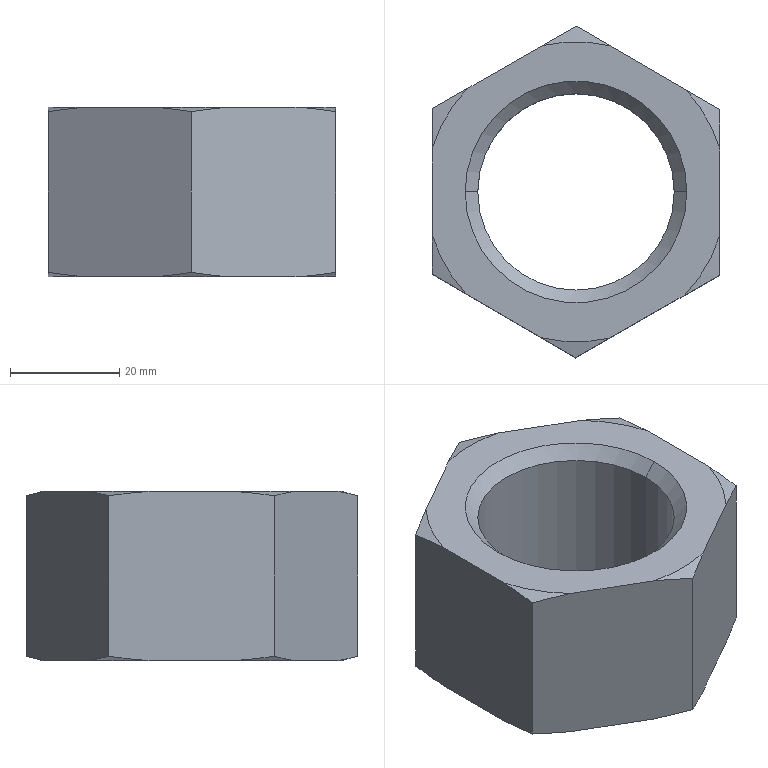Part | SolidWorks | features Cut 2, Chamfer 1, Extrusion 1 | 1 solid | 26 faces | box 52.765 x 60.79 x 31 mm | volume 42176 mm3 | cone 16 | plane 8 | cylinder 2 | commonest cylinder face diameters 36 x2
STEP:
#1=CARTESIAN_POINT('',(-18.,0.,28.693));
#2=VERTEX_POINT('',#1);
#3=CARTESIAN_POINT('',(18.,0.,28.693));
#4=VERTEX_POINT('',#3);
#5=CARTESIAN_POINT('',(0.,0.,28.693));
#6=DIRECTION('',(0.,0.,1.));
#7=DIRECTION('',(-1.,0.,0.));
#8=AXIS2_PLACEMENT_3D('',#5,#6,#7);
#9=CIRCLE('',#8,18.);
#10=EDGE_CURVE('',#2,#4,#9,.T.);
#11=ORIENTED_EDGE('',*,*,#10,.F.);
#12=CARTESIAN_POINT('',(-20.307,0.,31.));
#13=VERTEX_POINT('',#12);
#14=CARTESIAN_POINT('',(-18.,0.,28.693));
#15=DIRECTION('',(-0.7071,0.,0.7071));
#16=VECTOR('',#15,1000.);
#17=LINE('',#14,#16);
#18=EDGE_CURVE('',#2,#13,#17,.T.);
#19=ORIENTED_EDGE('',*,*,#18,.T.);
#20=CARTESIAN_POINT('',(20.307,0.,31.));
#21=VERTEX_POINT('',#20);
#22=CARTESIAN_POINT('',(0.,0.,31.));
#23=DIRECTION('',(0.,0.,-1.));
#24=DIRECTION('',(-1.,0.,0.));
#25=AXIS2_PLACEMENT_3D('',#22,#23,#24);
#26=CIRCLE('',#25,20.307);
#27=EDGE_CURVE('',#21,#13,#26,.T.);
#28=ORIENTED_EDGE('',*,*,#27,.F.);
#29=CARTESIAN_POINT('',(18.,0.,28.693));
#30=DIRECTION('',(0.7071,0.,0.7071));
#31=VECTOR('',#30,1000.);
#32=LINE('',#29,#31);
#33=EDGE_CURVE('',#4,#21,#32,.T.);
#34=ORIENTED_EDGE('',*,*,#33,.F.);
#35=EDGE_LOOP('',(#11,#19,#28,#34));
#36=FACE_OUTER_BOUND('',#35,.T.);
#37=CARTESIAN_POINT('',(0.,0.,28.693));
#38=DIRECTION('',(0.,0.,1.));
#39=DIRECTION('',(1.,0.,0.));
#40=AXIS2_PLACEMENT_3D('',#37,#38,#39);
#41=CONICAL_SURFACE('',#40,18.,0.7854);
#42=ADVANCED_FACE('',(#36),#41,.F.);
#43=CARTESIAN_POINT('',(18.,0.,2.307));
#44=VERTEX_POINT('',#43);
#45=CARTESIAN_POINT('',(-18.,0.,2.307));
#46=VERTEX_POINT('',#45);
#47=CARTESIAN_POINT('',(0.,0.,2.307));
#48=DIRECTION('',(0.,0.,-1.));
#49=DIRECTION('',(-1.,0.,0.));
#50=AXIS2_PLACEMENT_3D('',#47,#48,#49);
#51=CIRCLE('',#50,18.);
#52=EDGE_CURVE('',#44,#46,#51,.T.);
#53=ORIENTED_EDGE('',*,*,#52,.F.);
#54=CARTESIAN_POINT('',(20.307,0.,0.));
#55=VERTEX_POINT('',#54);
#56=CARTESIAN_POINT('',(20.307,0.,0.));
#57=DIRECTION('',(0.7071,0.,-0.7071));
#58=VECTOR('',#57,1000.);
#59=LINE('',#56,#58);
#60=EDGE_CURVE('',#44,#55,#59,.T.);
#61=ORIENTED_EDGE('',*,*,#60,.T.);
#62=CARTESIAN_POINT('',(-20.307,0.,0.));
#63=VERTEX_POINT('',#62);
#64=CARTESIAN_POINT('',(0.,0.,0.));
#65=DIRECTION('',(0.,0.,1.));
#66=DIRECTION('',(-1.,0.,0.));
#67=AXIS2_PLACEMENT_3D('',#64,#65,#66);
#68=CIRCLE('',#67,20.307);
#69=EDGE_CURVE('',#63,#55,#68,.T.);
#70=ORIENTED_EDGE('',*,*,#69,.F.);
#71=CARTESIAN_POINT('',(-20.307,0.,0.));
#72=DIRECTION('',(-0.7071,0.,-0.7071));
#73=VECTOR('',#72,1000.);
#74=LINE('',#71,#73);
#75=EDGE_CURVE('',#46,#63,#74,.T.);
#76=ORIENTED_EDGE('',*,*,#75,.F.);
#77=EDGE_LOOP('',(#53,#61,#70,#76));
#78=FACE_OUTER_BOUND('',#77,.T.);
#79=CARTESIAN_POINT('',(0.,0.,0.));
#80=DIRECTION('',(0.,0.,-1.));
#81=DIRECTION('',(-1.,0.,0.));
#82=AXIS2_PLACEMENT_3D('',#79,#80,#81);
#83=CONICAL_SURFACE('',#82,20.307,0.7854);
#84=ADVANCED_FACE('',(#78),#83,.F.);
#85=ORIENTED_EDGE('',*,*,#10,.T.);
#86=CARTESIAN_POINT('',(18.,0.,31.));
#87=DIRECTION('',(0.,0.,-1.));
#88=VECTOR('',#87,1000.);
#89=LINE('',#86,#88);
#90=EDGE_CURVE('',#4,#44,#89,.T.);
#91=ORIENTED_EDGE('',*,*,#90,.T.);
#92=ORIENTED_EDGE('',*,*,#52,.T.);
#93=CARTESIAN_POINT('',(-18.,0.,31.));
#94=DIRECTION('',(0.,0.,-1.));
#95=VECTOR('',#94,1000.);
#96=LINE('',#93,#95);
#97=EDGE_CURVE('',#2,#46,#96,.T.);
#98=ORIENTED_EDGE('',*,*,#97,.F.);
#99=EDGE_LOOP('',(#85,#91,#92,#98));
#100=FACE_OUTER_BOUND('',#99,.T.);
#101=CARTESIAN_POINT('',(0.,0.,31.));
#102=DIRECTION('',(0.,0.,-1.));
#103=DIRECTION('',(-1.,0.,0.));
#104=AXIS2_PLACEMENT_3D('',#101,#102,#103);
#105=CYLINDRICAL_SURFACE('',#104,18.);
#106=ADVANCED_FACE('',(#100),#105,.F.);
#107=CARTESIAN_POINT('',(26.382,15.094,30.224));
#108=VERTEX_POINT('',#107);
#109=CARTESIAN_POINT('',(20.129,18.737,31.));
#110=VERTEX_POINT('',#109);
#111=CARTESIAN_POINT('',(26.382,15.094,30.224));
#112=CARTESIAN_POINT('',(24.305,16.304,30.546));
#113=CARTESIAN_POINT('',(22.221,17.518,30.812));
#114=CARTESIAN_POINT('',(20.129,18.737,31.));
#115=B_SPLINE_CURVE_WITH_KNOTS('',3,(#111,#112,#113,#114),.UNSPECIFIED.,.F.,.F.,(4,4),(0.03012,0.0374),.UNSPECIFIED.);
#116=EDGE_CURVE('',#108,#110,#115,.T.);
#117=ORIENTED_EDGE('',*,*,#116,.F.);
#118=CARTESIAN_POINT('',(26.382,15.094,0.7757));
#119=VERTEX_POINT('',#118);
#120=CARTESIAN_POINT('',(26.382,15.094,31.));
#121=DIRECTION('',(0.,0.,-1.));
#122=VECTOR('',#121,1000.);
#123=LINE('',#120,#122);
#124=EDGE_CURVE('',#108,#119,#123,.T.);
#125=ORIENTED_EDGE('',*,*,#124,.T.);
#126=CARTESIAN_POINT('',(20.129,18.737,0.));
#127=VERTEX_POINT('',#126);
#128=CARTESIAN_POINT('',(20.129,18.737,0.));
#129=CARTESIAN_POINT('',(22.224,17.517,0.1881));
#130=CARTESIAN_POINT('',(24.308,16.303,0.454));
#131=CARTESIAN_POINT('',(26.382,15.094,0.7757));
#132=B_SPLINE_CURVE_WITH_KNOTS('',3,(#128,#129,#130,#131),.UNSPECIFIED.,.F.,.F.,(4,4),(0.0532,0.06035),.UNSPECIFIED.);
#133=EDGE_CURVE('',#127,#119,#132,.T.);
#134=ORIENTED_EDGE('',*,*,#133,.F.);
#135=CARTESIAN_POINT('',(6.373,26.751,0.));
#136=VERTEX_POINT('',#135);
#137=CARTESIAN_POINT('',(26.382,15.094,0.));
#138=DIRECTION('',(-0.8641,0.5034,0.));
#139=VECTOR('',#138,1000.);
#140=LINE('',#137,#139);
#141=EDGE_CURVE('',#127,#136,#140,.T.);
#142=ORIENTED_EDGE('',*,*,#141,.T.);
#143=CARTESIAN_POINT('',(0.1196,30.395,0.7757));
#144=VERTEX_POINT('',#143);
#145=CARTESIAN_POINT('',(0.1196,30.395,0.7757));
#146=CARTESIAN_POINT('',(2.197,29.184,0.4535));
#147=CARTESIAN_POINT('',(4.281,27.97,0.1878));
#148=CARTESIAN_POINT('',(6.373,26.751,0.));
#149=B_SPLINE_CURVE_WITH_KNOTS('',3,(#145,#146,#147,#148),.UNSPECIFIED.,.F.,.F.,(4,4),(0.03012,0.0374),.UNSPECIFIED.);
#150=EDGE_CURVE('',#144,#136,#149,.T.);
#151=ORIENTED_EDGE('',*,*,#150,.F.);
#152=CARTESIAN_POINT('',(0.1196,30.395,30.224));
#153=VERTEX_POINT('',#152);
#154=CARTESIAN_POINT('',(0.1196,30.395,31.));
#155=DIRECTION('',(0.,0.,-1.));
#156=VECTOR('',#155,1000.);
#157=LINE('',#154,#156);
#158=EDGE_CURVE('',#153,#144,#157,.T.);
#159=ORIENTED_EDGE('',*,*,#158,.F.);
#160=CARTESIAN_POINT('',(6.373,26.751,31.));
#161=VERTEX_POINT('',#160);
#162=CARTESIAN_POINT('',(6.373,26.751,31.));
#163=CARTESIAN_POINT('',(4.278,27.972,30.812));
#164=CARTESIAN_POINT('',(2.194,29.186,30.546));
#165=CARTESIAN_POINT('',(0.1196,30.395,30.224));
#166=B_SPLINE_CURVE_WITH_KNOTS('',3,(#162,#163,#164,#165),.UNSPECIFIED.,.F.,.F.,(4,4),(0.0532,0.06035),.UNSPECIFIED.);
#167=EDGE_CURVE('',#161,#153,#166,.T.);
#168=ORIENTED_EDGE('',*,*,#167,.F.);
#169=CARTESIAN_POINT('',(26.382,15.094,31.));
#170=DIRECTION('',(-0.8641,0.5034,0.));
#171=VECTOR('',#170,1000.);
#172=LINE('',#169,#171);
#173=EDGE_CURVE('',#110,#161,#172,.T.);
#174=ORIENTED_EDGE('',*,*,#173,.F.);
#175=EDGE_LOOP('',(#117,#125,#134,#142,#151,#159,#168,#174));
#176=FACE_OUTER_BOUND('',#175,.T.);
#177=CARTESIAN_POINT('',(26.382,15.094,31.));
#178=DIRECTION('',(-0.5034,-0.8641,0.));
#179=DIRECTION('',(0.8641,-0.5034,0.));
#180=AXIS2_PLACEMENT_3D('',#177,#178,#179);
#181=PLANE('',#180);
#182=ADVANCED_FACE('',(#176),#181,.F.);
#183=CARTESIAN_POINT('',(-6.163,26.801,31.));
#184=VERTEX_POINT('',#183);
#185=CARTESIAN_POINT('',(0.1196,30.395,30.224));
#186=CARTESIAN_POINT('',(-1.968,29.201,30.546));
#187=CARTESIAN_POINT('',(-4.061,28.003,30.812));
#188=CARTESIAN_POINT('',(-6.163,26.801,31.));
#189=B_SPLINE_CURVE_WITH_KNOTS('',3,(#185,#186,#187,#188),.UNSPECIFIED.,.F.,.F.,(4,4),(0.02999,0.03726),.UNSPECIFIED.);
#190=EDGE_CURVE('',#153,#184,#189,.T.);
#191=ORIENTED_EDGE('',*,*,#190,.F.);
#192=ORIENTED_EDGE('',*,*,#158,.T.);
#193=CARTESIAN_POINT('',(-6.163,26.801,0.));
#194=VERTEX_POINT('',#193);
#195=CARTESIAN_POINT('',(-6.163,26.801,0.));
#196=CARTESIAN_POINT('',(-4.058,28.005,0.1881));
#197=CARTESIAN_POINT('',(-1.965,29.202,0.454));
#198=CARTESIAN_POINT('',(0.1196,30.395,0.7757));
#199=B_SPLINE_CURVE_WITH_KNOTS('',3,(#195,#196,#197,#198),.UNSPECIFIED.,.F.,.F.,(4,4),(0.05306,0.06021),.UNSPECIFIED.);
#200=EDGE_CURVE('',#194,#144,#199,.T.);
#201=ORIENTED_EDGE('',*,*,#200,.F.);
#202=CARTESIAN_POINT('',(-19.981,18.895,0.));
#203=VERTEX_POINT('',#202);
#204=CARTESIAN_POINT('',(0.1196,30.395,0.));
#205=DIRECTION('',(-0.868,-0.4966,0.));
#206=VECTOR('',#205,1000.);
#207=LINE('',#204,#206);
#208=EDGE_CURVE('',#194,#203,#207,.T.);
#209=ORIENTED_EDGE('',*,*,#208,.T.);
#210=CARTESIAN_POINT('',(-26.263,15.301,0.7757));
#211=VERTEX_POINT('',#210);
#212=CARTESIAN_POINT('',(-26.263,15.301,0.7757));
#213=CARTESIAN_POINT('',(-24.176,16.495,0.4535));
#214=CARTESIAN_POINT('',(-22.082,17.693,0.1878));
#215=CARTESIAN_POINT('',(-19.981,18.895,0.));
#216=B_SPLINE_CURVE_WITH_KNOTS('',3,(#212,#213,#214,#215),.UNSPECIFIED.,.F.,.F.,(4,4),(0.02999,0.03726),.UNSPECIFIED.);
#217=EDGE_CURVE('',#211,#203,#216,.T.);
#218=ORIENTED_EDGE('',*,*,#217,.F.);
#219=CARTESIAN_POINT('',(-26.263,15.301,30.224));
#220=VERTEX_POINT('',#219);
#221=CARTESIAN_POINT('',(-26.263,15.301,31.));
#222=DIRECTION('',(0.,0.,-1.));
#223=VECTOR('',#222,1000.);
#224=LINE('',#221,#223);
#225=EDGE_CURVE('',#220,#211,#224,.T.);
#226=ORIENTED_EDGE('',*,*,#225,.F.);
#227=CARTESIAN_POINT('',(-19.981,18.895,31.));
#228=VERTEX_POINT('',#227);
#229=CARTESIAN_POINT('',(-19.981,18.895,31.));
#230=CARTESIAN_POINT('',(-22.086,17.691,30.812));
#231=CARTESIAN_POINT('',(-24.179,16.493,30.546));
#232=CARTESIAN_POINT('',(-26.263,15.301,30.224));
#233=B_SPLINE_CURVE_WITH_KNOTS('',3,(#229,#230,#231,#232),.UNSPECIFIED.,.F.,.F.,(4,4),(0.05306,0.06021),.UNSPECIFIED.);
#234=EDGE_CURVE('',#228,#220,#233,.T.);
#235=ORIENTED_EDGE('',*,*,#234,.F.);
#236=CARTESIAN_POINT('',(0.1196,30.395,31.));
#237=DIRECTION('',(-0.868,-0.4966,0.));
#238=VECTOR('',#237,1000.);
#239=LINE('',#236,#238);
#240=EDGE_CURVE('',#184,#228,#239,.T.);
#241=ORIENTED_EDGE('',*,*,#240,.F.);
#242=EDGE_LOOP('',(#191,#192,#201,#209,#218,#226,#235,#241));
#243=FACE_OUTER_BOUND('',#242,.T.);
#244=CARTESIAN_POINT('',(0.1196,30.395,31.));
#245=DIRECTION('',(0.4966,-0.868,0.));
#246=DIRECTION('',(0.868,0.4966,0.));
#247=AXIS2_PLACEMENT_3D('',#244,#245,#246);
#248=PLANE('',#247);
#249=ADVANCED_FACE('',(#243),#248,.F.);
#250=CARTESIAN_POINT('',(-26.291,8.063,31.));
#251=VERTEX_POINT('',#250);
#252=CARTESIAN_POINT('',(-26.263,15.301,30.224));
#253=CARTESIAN_POINT('',(-26.272,12.896,30.547));
#254=CARTESIAN_POINT('',(-26.282,10.484,30.812));
#255=CARTESIAN_POINT('',(-26.291,8.063,31.));
#256=B_SPLINE_CURVE_WITH_KNOTS('',3,(#252,#253,#254,#255),.UNSPECIFIED.,.F.,.F.,(4,4),(0.02599,0.03327),.UNSPECIFIED.);
#257=EDGE_CURVE('',#220,#251,#256,.T.);
#258=ORIENTED_EDGE('',*,*,#257,.F.);
#259=ORIENTED_EDGE('',*,*,#225,.T.);
#260=CARTESIAN_POINT('',(-26.291,8.063,0.));
#261=VERTEX_POINT('',#260);
#262=CARTESIAN_POINT('',(-26.291,8.063,0.));
#263=CARTESIAN_POINT('',(-26.287,9.274,0.09389));
#264=CARTESIAN_POINT('',(-26.282,10.484,0.2075));
#265=CARTESIAN_POINT('',(-26.272,12.897,0.4679));
#266=CARTESIAN_POINT('',(-26.268,14.1,0.6148));
#267=CARTESIAN_POINT('',(-26.263,15.301,0.7757));
#268=B_SPLINE_CURVE_WITH_KNOTS('',3,(#262,#263,#264,#265,#266,#267),.UNSPECIFIED.,.F.,.F.,(4,2,4),(0.04909,0.05267,0.05624),.UNSPECIFIED.);
#269=EDGE_CURVE('',#261,#211,#268,.T.);
#270=ORIENTED_EDGE('',*,*,#269,.F.);
#271=CARTESIAN_POINT('',(-26.354,-7.856,0.));
#272=VERTEX_POINT('',#271);
#273=CARTESIAN_POINT('',(-26.263,15.301,0.));
#274=DIRECTION('',(-0.003934,-1.,0.));
#275=VECTOR('',#274,1000.);
#276=LINE('',#273,#275);
#277=EDGE_CURVE('',#261,#272,#276,.T.);
#278=ORIENTED_EDGE('',*,*,#277,.T.);
#279=CARTESIAN_POINT('',(-26.382,-15.094,0.7757));
#280=VERTEX_POINT('',#279);
#281=CARTESIAN_POINT('',(-26.382,-15.094,0.7757));
#282=CARTESIAN_POINT('',(-26.373,-12.688,0.4535));
#283=CARTESIAN_POINT('',(-26.363,-10.277,0.1877));
#284=CARTESIAN_POINT('',(-26.354,-7.856,0.));
#285=B_SPLINE_CURVE_WITH_KNOTS('',3,(#281,#282,#283,#284),.UNSPECIFIED.,.F.,.F.,(4,4),(0.02599,0.03327),.UNSPECIFIED.);
#286=EDGE_CURVE('',#280,#272,#285,.T.);
#287=ORIENTED_EDGE('',*,*,#286,.F.);
#288=CARTESIAN_POINT('',(-26.382,-15.094,30.224));
#289=VERTEX_POINT('',#288);
#290=CARTESIAN_POINT('',(-26.382,-15.094,31.));
#291=DIRECTION('',(0.,0.,-1.));
#292=VECTOR('',#291,1000.);
#293=LINE('',#290,#292);
#294=EDGE_CURVE('',#289,#280,#293,.T.);
#295=ORIENTED_EDGE('',*,*,#294,.F.);
#296=CARTESIAN_POINT('',(-26.354,-7.856,31.));
#297=VERTEX_POINT('',#296);
#298=CARTESIAN_POINT('',(-26.354,-7.856,31.));
#299=CARTESIAN_POINT('',(-26.359,-9.067,30.906));
#300=CARTESIAN_POINT('',(-26.363,-10.277,30.793));
#301=CARTESIAN_POINT('',(-26.373,-12.69,30.532));
#302=CARTESIAN_POINT('',(-26.378,-13.893,30.385));
#303=CARTESIAN_POINT('',(-26.382,-15.094,30.224));
#304=B_SPLINE_CURVE_WITH_KNOTS('',3,(#298,#299,#300,#301,#302,#303),.UNSPECIFIED.,.F.,.F.,(4,2,4),(0.04909,0.05267,0.05624),.UNSPECIFIED.);
#305=EDGE_CURVE('',#297,#289,#304,.T.);
#306=ORIENTED_EDGE('',*,*,#305,.F.);
#307=CARTESIAN_POINT('',(-26.263,15.301,31.));
#308=DIRECTION('',(-0.003934,-1.,0.));
#309=VECTOR('',#308,1000.);
#310=LINE('',#307,#309);
#311=EDGE_CURVE('',#251,#297,#310,.T.);
#312=ORIENTED_EDGE('',*,*,#311,.F.);
#313=EDGE_LOOP('',(#258,#259,#270,#278,#287,#295,#306,#312));
#314=FACE_OUTER_BOUND('',#313,.T.);
#315=CARTESIAN_POINT('',(-26.263,15.301,31.));
#316=DIRECTION('',(1.,-0.003934,0.));
#317=DIRECTION('',(0.003934,1.,0.));
#318=AXIS2_PLACEMENT_3D('',#315,#316,#317);
#319=PLANE('',#318);
#320=ADVANCED_FACE('',(#314),#319,.F.);
#321=CARTESIAN_POINT('',(-20.129,-18.737,31.));
#322=VERTEX_POINT('',#321);
#323=CARTESIAN_POINT('',(-26.382,-15.094,30.224));
#324=CARTESIAN_POINT('',(-24.305,-16.304,30.546));
#325=CARTESIAN_POINT('',(-22.221,-17.518,30.812));
#326=CARTESIAN_POINT('',(-20.129,-18.737,31.));
#327=B_SPLINE_CURVE_WITH_KNOTS('',3,(#323,#324,#325,#326),.UNSPECIFIED.,.F.,.F.,(4,4),(0.03012,0.0374),.UNSPECIFIED.);
#328=EDGE_CURVE('',#289,#322,#327,.T.);
#329=ORIENTED_EDGE('',*,*,#328,.F.);
#330=ORIENTED_EDGE('',*,*,#294,.T.);
#331=CARTESIAN_POINT('',(-20.129,-18.737,0.));
#332=VERTEX_POINT('',#331);
#333=CARTESIAN_POINT('',(-20.129,-18.737,0.));
#334=CARTESIAN_POINT('',(-22.224,-17.517,0.1881));
#335=CARTESIAN_POINT('',(-24.308,-16.303,0.454));
#336=CARTESIAN_POINT('',(-26.382,-15.094,0.7757));
#337=B_SPLINE_CURVE_WITH_KNOTS('',3,(#333,#334,#335,#336),.UNSPECIFIED.,.F.,.F.,(4,4),(0.0532,0.06035),.UNSPECIFIED.);
#338=EDGE_CURVE('',#332,#280,#337,.T.);
#339=ORIENTED_EDGE('',*,*,#338,.F.);
#340=CARTESIAN_POINT('',(-6.373,-26.751,0.));
#341=VERTEX_POINT('',#340);
#342=CARTESIAN_POINT('',(-26.382,-15.094,0.));
#343=DIRECTION('',(0.8641,-0.5034,0.));
#344=VECTOR('',#343,1000.);
#345=LINE('',#342,#344);
#346=EDGE_CURVE('',#332,#341,#345,.T.);
#347=ORIENTED_EDGE('',*,*,#346,.T.);
#348=CARTESIAN_POINT('',(-0.1196,-30.395,0.7757));
#349=VERTEX_POINT('',#348);
#350=CARTESIAN_POINT('',(-0.1196,-30.395,0.7757));
#351=CARTESIAN_POINT('',(-2.197,-29.184,0.4535));
#352=CARTESIAN_POINT('',(-4.281,-27.97,0.1878));
#353=CARTESIAN_POINT('',(-6.373,-26.751,0.));
#354=B_SPLINE_CURVE_WITH_KNOTS('',3,(#350,#351,#352,#353),.UNSPECIFIED.,.F.,.F.,(4,4),(0.03012,0.0374),.UNSPECIFIED.);
#355=EDGE_CURVE('',#349,#341,#354,.T.);
#356=ORIENTED_EDGE('',*,*,#355,.F.);
#357=CARTESIAN_POINT('',(-0.1196,-30.395,30.224));
#358=VERTEX_POINT('',#357);
#359=CARTESIAN_POINT('',(-0.1196,-30.395,31.));
#360=DIRECTION('',(0.,0.,-1.));
#361=VECTOR('',#360,1000.);
#362=LINE('',#359,#361);
#363=EDGE_CURVE('',#358,#349,#362,.T.);
#364=ORIENTED_EDGE('',*,*,#363,.F.);
#365=CARTESIAN_POINT('',(-6.373,-26.751,31.));
#366=VERTEX_POINT('',#365);
#367=CARTESIAN_POINT('',(-6.373,-26.751,31.));
#368=CARTESIAN_POINT('',(-4.278,-27.972,30.812));
#369=CARTESIAN_POINT('',(-2.194,-29.186,30.546));
#370=CARTESIAN_POINT('',(-0.1196,-30.395,30.224));
#371=B_SPLINE_CURVE_WITH_KNOTS('',3,(#367,#368,#369,#370),.UNSPECIFIED.,.F.,.F.,(4,4),(0.0532,0.06035),.UNSPECIFIED.);
#372=EDGE_CURVE('',#366,#358,#371,.T.);
#373=ORIENTED_EDGE('',*,*,#372,.F.);
#374=CARTESIAN_POINT('',(-26.382,-15.094,31.));
#375=DIRECTION('',(0.8641,-0.5034,0.));
#376=VECTOR('',#375,1000.);
#377=LINE('',#374,#376);
#378=EDGE_CURVE('',#322,#366,#377,.T.);
#379=ORIENTED_EDGE('',*,*,#378,.F.);
#380=EDGE_LOOP('',(#329,#330,#339,#347,#356,#364,#373,#379));
#381=FACE_OUTER_BOUND('',#380,.T.);
#382=CARTESIAN_POINT('',(-26.382,-15.094,31.));
#383=DIRECTION('',(0.5034,0.8641,0.));
#384=DIRECTION('',(-0.8641,0.5034,0.));
#385=AXIS2_PLACEMENT_3D('',#382,#383,#384);
#386=PLANE('',#385);
#387=ADVANCED_FACE('',(#381),#386,.F.);
#388=CARTESIAN_POINT('',(6.163,-26.801,31.));
#389=VERTEX_POINT('',#388);
#390=CARTESIAN_POINT('',(-0.1196,-30.395,30.224));
#391=CARTESIAN_POINT('',(1.968,-29.201,30.546));
#392=CARTESIAN_POINT('',(4.061,-28.003,30.812));
#393=CARTESIAN_POINT('',(6.163,-26.801,31.));
#394=B_SPLINE_CURVE_WITH_KNOTS('',3,(#390,#391,#392,#393),.UNSPECIFIED.,.F.,.F.,(4,4),(0.02999,0.03726),.UNSPECIFIED.);
#395=EDGE_CURVE('',#358,#389,#394,.T.);
#396=ORIENTED_EDGE('',*,*,#395,.F.);
#397=ORIENTED_EDGE('',*,*,#363,.T.);
#398=CARTESIAN_POINT('',(6.163,-26.801,0.));
#399=VERTEX_POINT('',#398);
#400=CARTESIAN_POINT('',(6.163,-26.801,0.));
#401=CARTESIAN_POINT('',(4.058,-28.005,0.1881));
#402=CARTESIAN_POINT('',(1.965,-29.202,0.454));
#403=CARTESIAN_POINT('',(-0.1196,-30.395,0.7757));
#404=B_SPLINE_CURVE_WITH_KNOTS('',3,(#400,#401,#402,#403),.UNSPECIFIED.,.F.,.F.,(4,4),(0.05306,0.06021),.UNSPECIFIED.);
#405=EDGE_CURVE('',#399,#349,#404,.T.);
#406=ORIENTED_EDGE('',*,*,#405,.F.);
#407=CARTESIAN_POINT('',(19.981,-18.895,0.));
#408=VERTEX_POINT('',#407);
#409=CARTESIAN_POINT('',(-0.1196,-30.395,0.));
#410=DIRECTION('',(0.868,0.4966,0.));
#411=VECTOR('',#410,1000.);
#412=LINE('',#409,#411);
#413=EDGE_CURVE('',#399,#408,#412,.T.);
#414=ORIENTED_EDGE('',*,*,#413,.T.);
#415=CARTESIAN_POINT('',(26.263,-15.301,0.7757));
#416=VERTEX_POINT('',#415);
#417=CARTESIAN_POINT('',(26.263,-15.301,0.7757));
#418=CARTESIAN_POINT('',(24.176,-16.495,0.4535));
#419=CARTESIAN_POINT('',(22.082,-17.693,0.1878));
#420=CARTESIAN_POINT('',(19.981,-18.895,0.));
#421=B_SPLINE_CURVE_WITH_KNOTS('',3,(#417,#418,#419,#420),.UNSPECIFIED.,.F.,.F.,(4,4),(0.02999,0.03726),.UNSPECIFIED.);
#422=EDGE_CURVE('',#416,#408,#421,.T.);
#423=ORIENTED_EDGE('',*,*,#422,.F.);
#424=CARTESIAN_POINT('',(26.263,-15.301,30.224));
#425=VERTEX_POINT('',#424);
#426=CARTESIAN_POINT('',(26.263,-15.301,31.));
#427=DIRECTION('',(0.,0.,-1.));
#428=VECTOR('',#427,1000.);
#429=LINE('',#426,#428);
#430=EDGE_CURVE('',#425,#416,#429,.T.);
#431=ORIENTED_EDGE('',*,*,#430,.F.);
#432=CARTESIAN_POINT('',(19.981,-18.895,31.));
#433=VERTEX_POINT('',#432);
#434=CARTESIAN_POINT('',(19.981,-18.895,31.));
#435=CARTESIAN_POINT('',(22.086,-17.691,30.812));
#436=CARTESIAN_POINT('',(24.179,-16.493,30.546));
#437=CARTESIAN_POINT('',(26.263,-15.301,30.224));
#438=B_SPLINE_CURVE_WITH_KNOTS('',3,(#434,#435,#436,#437),.UNSPECIFIED.,.F.,.F.,(4,4),(0.05306,0.06021),.UNSPECIFIED.);
#439=EDGE_CURVE('',#433,#425,#438,.T.);
#440=ORIENTED_EDGE('',*,*,#439,.F.);
#441=CARTESIAN_POINT('',(-0.1196,-30.395,31.));
#442=DIRECTION('',(0.868,0.4966,0.));
#443=VECTOR('',#442,1000.);
#444=LINE('',#441,#443);
#445=EDGE_CURVE('',#389,#433,#444,.T.);
#446=ORIENTED_EDGE('',*,*,#445,.F.);
#447=EDGE_LOOP('',(#396,#397,#406,#414,#423,#431,#440,#446));
#448=FACE_OUTER_BOUND('',#447,.T.);
#449=CARTESIAN_POINT('',(-0.1196,-30.395,31.));
#450=DIRECTION('',(-0.4966,0.868,0.));
#451=DIRECTION('',(-0.868,-0.4966,0.));
#452=AXIS2_PLACEMENT_3D('',#449,#450,#451);
#453=PLANE('',#452);
#454=ADVANCED_FACE('',(#448),#453,.F.);
#455=CARTESIAN_POINT('',(26.291,-8.063,31.));
#456=VERTEX_POINT('',#455);
#457=CARTESIAN_POINT('',(26.263,-15.301,30.224));
#458=CARTESIAN_POINT('',(26.272,-12.896,30.547));
#459=CARTESIAN_POINT('',(26.282,-10.484,30.812));
#460=CARTESIAN_POINT('',(26.291,-8.063,31.));
#461=B_SPLINE_CURVE_WITH_KNOTS('',3,(#457,#458,#459,#460),.UNSPECIFIED.,.F.,.F.,(4,4),(0.02599,0.03327),.UNSPECIFIED.);
#462=EDGE_CURVE('',#425,#456,#461,.T.);
#463=ORIENTED_EDGE('',*,*,#462,.F.);
#464=ORIENTED_EDGE('',*,*,#430,.T.);
#465=CARTESIAN_POINT('',(26.291,-8.063,0.));
#466=VERTEX_POINT('',#465);
#467=CARTESIAN_POINT('',(26.291,-8.063,0.));
#468=CARTESIAN_POINT('',(26.287,-9.274,0.09389));
#469=CARTESIAN_POINT('',(26.282,-10.484,0.2075));
#470=CARTESIAN_POINT('',(26.272,-12.897,0.4679));
#471=CARTESIAN_POINT('',(26.268,-14.1,0.6148));
#472=CARTESIAN_POINT('',(26.263,-15.301,0.7757));
#473=B_SPLINE_CURVE_WITH_KNOTS('',3,(#467,#468,#469,#470,#471,#472),.UNSPECIFIED.,.F.,.F.,(4,2,4),(0.04909,0.05267,0.05624),.UNSPECIFIED.);
#474=EDGE_CURVE('',#466,#416,#473,.T.);
#475=ORIENTED_EDGE('',*,*,#474,.F.);
#476=CARTESIAN_POINT('',(26.354,7.856,0.));
#477=VERTEX_POINT('',#476);
#478=CARTESIAN_POINT('',(26.263,-15.301,0.));
#479=DIRECTION('',(0.003934,1.,0.));
#480=VECTOR('',#479,1000.);
#481=LINE('',#478,#480);
#482=EDGE_CURVE('',#466,#477,#481,.T.);
#483=ORIENTED_EDGE('',*,*,#482,.T.);
#484=CARTESIAN_POINT('',(26.382,15.094,0.7757));
#485=CARTESIAN_POINT('',(26.373,12.688,0.4535));
#486=CARTESIAN_POINT('',(26.363,10.277,0.1877));
#487=CARTESIAN_POINT('',(26.354,7.856,0.));
#488=B_SPLINE_CURVE_WITH_KNOTS('',3,(#484,#485,#486,#487),.UNSPECIFIED.,.F.,.F.,(4,4),(0.02599,0.03327),.UNSPECIFIED.);
#489=EDGE_CURVE('',#119,#477,#488,.T.);
#490=ORIENTED_EDGE('',*,*,#489,.F.);
#491=ORIENTED_EDGE('',*,*,#124,.F.);
#492=CARTESIAN_POINT('',(26.354,7.856,31.));
#493=VERTEX_POINT('',#492);
#494=CARTESIAN_POINT('',(26.354,7.856,31.));
#495=CARTESIAN_POINT('',(26.359,9.067,30.906));
#496=CARTESIAN_POINT('',(26.363,10.277,30.793));
#497=CARTESIAN_POINT('',(26.373,12.69,30.532));
#498=CARTESIAN_POINT('',(26.378,13.893,30.385));
#499=CARTESIAN_POINT('',(26.382,15.094,30.224));
#500=B_SPLINE_CURVE_WITH_KNOTS('',3,(#494,#495,#496,#497,#498,#499),.UNSPECIFIED.,.F.,.F.,(4,2,4),(0.04909,0.05267,0.05624),.UNSPECIFIED.);
#501=EDGE_CURVE('',#493,#108,#500,.T.);
#502=ORIENTED_EDGE('',*,*,#501,.F.);
#503=CARTESIAN_POINT('',(26.263,-15.301,31.));
#504=DIRECTION('',(0.003934,1.,0.));
#505=VECTOR('',#504,1000.);
#506=LINE('',#503,#505);
#507=EDGE_CURVE('',#456,#493,#506,.T.);
#508=ORIENTED_EDGE('',*,*,#507,.F.);
#509=EDGE_LOOP('',(#463,#464,#475,#483,#490,#491,#502,#508));
#510=FACE_OUTER_BOUND('',#509,.T.);
#511=CARTESIAN_POINT('',(26.263,-15.301,31.));
#512=DIRECTION('',(-1.,0.003934,0.));
#513=DIRECTION('',(-0.003934,-1.,0.));
#514=AXIS2_PLACEMENT_3D('',#511,#512,#513);
#515=PLANE('',#514);
#516=ADVANCED_FACE('',(#510),#515,.F.);
#517=ORIENTED_EDGE('',*,*,#27,.T.);
#518=CARTESIAN_POINT('',(0.,0.,31.));
#519=DIRECTION('',(0.,0.,-1.));
#520=DIRECTION('',(-1.,0.,0.));
#521=AXIS2_PLACEMENT_3D('',#518,#519,#520);
#522=CIRCLE('',#521,20.307);
#523=EDGE_CURVE('',#13,#21,#522,.T.);
#524=ORIENTED_EDGE('',*,*,#523,.T.);
#525=EDGE_LOOP('',(#517,#524));
#526=FACE_BOUND('',#525,.T.);
#527=CARTESIAN_POINT('',(0.,0.,31.));
#528=DIRECTION('',(0.,0.,-1.));
#529=DIRECTION('',(-1.,0.,0.));
#530=AXIS2_PLACEMENT_3D('',#527,#528,#529);
#531=CIRCLE('',#530,27.5);
#532=EDGE_CURVE('',#251,#228,#531,.T.);
#533=ORIENTED_EDGE('',*,*,#532,.F.);
#534=ORIENTED_EDGE('',*,*,#311,.T.);
#535=CARTESIAN_POINT('',(0.,0.,31.));
#536=DIRECTION('',(0.,0.,-1.));
#537=DIRECTION('',(-1.,0.,0.));
#538=AXIS2_PLACEMENT_3D('',#535,#536,#537);
#539=CIRCLE('',#538,27.5);
#540=EDGE_CURVE('',#322,#297,#539,.T.);
#541=ORIENTED_EDGE('',*,*,#540,.F.);
#542=ORIENTED_EDGE('',*,*,#378,.T.);
#543=CARTESIAN_POINT('',(0.,0.,31.));
#544=DIRECTION('',(0.,0.,-1.));
#545=DIRECTION('',(-1.,0.,0.));
#546=AXIS2_PLACEMENT_3D('',#543,#544,#545);
#547=CIRCLE('',#546,27.5);
#548=EDGE_CURVE('',#389,#366,#547,.T.);
#549=ORIENTED_EDGE('',*,*,#548,.F.);
#550=ORIENTED_EDGE('',*,*,#445,.T.);
#551=CARTESIAN_POINT('',(0.,0.,31.));
#552=DIRECTION('',(0.,0.,-1.));
#553=DIRECTION('',(-1.,0.,0.));
#554=AXIS2_PLACEMENT_3D('',#551,#552,#553);
#555=CIRCLE('',#554,27.5);
#556=EDGE_CURVE('',#456,#433,#555,.T.);
#557=ORIENTED_EDGE('',*,*,#556,.F.);
#558=ORIENTED_EDGE('',*,*,#507,.T.);
#559=CARTESIAN_POINT('',(0.,0.,31.));
#560=DIRECTION('',(0.,0.,1.));
#561=DIRECTION('',(1.,0.,0.));
#562=AXIS2_PLACEMENT_3D('',#559,#560,#561);
#563=CIRCLE('',#562,27.5);
#564=EDGE_CURVE('',#493,#110,#563,.T.);
#565=ORIENTED_EDGE('',*,*,#564,.T.);
#566=ORIENTED_EDGE('',*,*,#173,.T.);
#567=CARTESIAN_POINT('',(0.,0.,31.));
#568=DIRECTION('',(0.,0.,-1.));
#569=DIRECTION('',(-1.,0.,0.));
#570=AXIS2_PLACEMENT_3D('',#567,#568,#569);
#571=CIRCLE('',#570,27.5);
#572=EDGE_CURVE('',#184,#161,#571,.T.);
#573=ORIENTED_EDGE('',*,*,#572,.F.);
#574=ORIENTED_EDGE('',*,*,#240,.T.);
#575=EDGE_LOOP('',(#533,#534,#541,#542,#549,#550,#557,#558,#565,#566,#573,#574));
#576=FACE_OUTER_BOUND('',#575,.T.);
#577=CARTESIAN_POINT('',(52.645,-0.2071,31.));
#578=DIRECTION('',(0.,0.,-1.));
#579=DIRECTION('',(-1.,0.,0.));
#580=AXIS2_PLACEMENT_3D('',#577,#578,#579);
#581=PLANE('',#580);
#582=ADVANCED_FACE('',(#526,#576),#581,.F.);
#583=ORIENTED_EDGE('',*,*,#69,.T.);
#584=CARTESIAN_POINT('',(0.,0.,0.));
#585=DIRECTION('',(0.,0.,1.));
#586=DIRECTION('',(-1.,0.,0.));
#587=AXIS2_PLACEMENT_3D('',#584,#585,#586);
#588=CIRCLE('',#587,20.307);
#589=EDGE_CURVE('',#55,#63,#588,.T.);
#590=ORIENTED_EDGE('',*,*,#589,.T.);
#591=EDGE_LOOP('',(#583,#590));
#592=FACE_BOUND('',#591,.T.);
#593=ORIENTED_EDGE('',*,*,#277,.F.);
#594=CARTESIAN_POINT('',(0.,0.,0.));
#595=DIRECTION('',(0.,0.,-1.));
#596=DIRECTION('',(-1.,0.,0.));
#597=AXIS2_PLACEMENT_3D('',#594,#595,#596);
#598=CIRCLE('',#597,27.5);
#599=EDGE_CURVE('',#261,#203,#598,.T.);
#600=ORIENTED_EDGE('',*,*,#599,.T.);
#601=ORIENTED_EDGE('',*,*,#208,.F.);
#602=CARTESIAN_POINT('',(0.,0.,0.));
#603=DIRECTION('',(0.,0.,-1.));
#604=DIRECTION('',(-1.,0.,0.));
#605=AXIS2_PLACEMENT_3D('',#602,#603,#604);
#606=CIRCLE('',#605,27.5);
#607=EDGE_CURVE('',#194,#136,#606,.T.);
#608=ORIENTED_EDGE('',*,*,#607,.T.);
#609=ORIENTED_EDGE('',*,*,#141,.F.);
#610=CARTESIAN_POINT('',(0.,0.,0.));
#611=DIRECTION('',(0.,0.,-1.));
#612=DIRECTION('',(-1.,0.,0.));
#613=AXIS2_PLACEMENT_3D('',#610,#611,#612);
#614=CIRCLE('',#613,27.5);
#615=EDGE_CURVE('',#127,#477,#614,.T.);
#616=ORIENTED_EDGE('',*,*,#615,.T.);
#617=ORIENTED_EDGE('',*,*,#482,.F.);
#618=CARTESIAN_POINT('',(0.,0.,0.));
#619=DIRECTION('',(0.,0.,-1.));
#620=DIRECTION('',(-1.,0.,0.));
#621=AXIS2_PLACEMENT_3D('',#618,#619,#620);
#622=CIRCLE('',#621,27.5);
#623=EDGE_CURVE('',#466,#408,#622,.T.);
#624=ORIENTED_EDGE('',*,*,#623,.T.);
#625=ORIENTED_EDGE('',*,*,#413,.F.);
#626=CARTESIAN_POINT('',(0.,0.,0.));
#627=DIRECTION('',(0.,0.,-1.));
#628=DIRECTION('',(-1.,0.,0.));
#629=AXIS2_PLACEMENT_3D('',#626,#627,#628);
#630=CIRCLE('',#629,27.5);
#631=EDGE_CURVE('',#399,#341,#630,.T.);
#632=ORIENTED_EDGE('',*,*,#631,.T.);
#633=ORIENTED_EDGE('',*,*,#346,.F.);
#634=CARTESIAN_POINT('',(0.,0.,0.));
#635=DIRECTION('',(0.,0.,-1.));
#636=DIRECTION('',(-1.,0.,0.));
#637=AXIS2_PLACEMENT_3D('',#634,#635,#636);
#638=CIRCLE('',#637,27.5);
#639=EDGE_CURVE('',#332,#272,#638,.T.);
#640=ORIENTED_EDGE('',*,*,#639,.T.);
#641=EDGE_LOOP('',(#593,#600,#601,#608,#609,#616,#617,#624,#625,#632,#633,#640));
#642=FACE_OUTER_BOUND('',#641,.T.);
#643=CARTESIAN_POINT('',(52.645,-0.2071,0.));
#644=DIRECTION('',(0.,0.,-1.));
#645=DIRECTION('',(-1.,0.,0.));
#646=AXIS2_PLACEMENT_3D('',#643,#644,#645);
#647=PLANE('',#646);
#648=ADVANCED_FACE('',(#592,#642),#647,.T.);
#649=ORIENTED_EDGE('',*,*,#90,.F.);
#650=CARTESIAN_POINT('',(0.,0.,28.693));
#651=DIRECTION('',(0.,0.,1.));
#652=DIRECTION('',(-1.,0.,0.));
#653=AXIS2_PLACEMENT_3D('',#650,#651,#652);
#654=CIRCLE('',#653,18.);
#655=EDGE_CURVE('',#4,#2,#654,.T.);
#656=ORIENTED_EDGE('',*,*,#655,.T.);
#657=ORIENTED_EDGE('',*,*,#97,.T.);
#658=CARTESIAN_POINT('',(0.,0.,2.307));
#659=DIRECTION('',(0.,0.,-1.));
#660=DIRECTION('',(-1.,0.,0.));
#661=AXIS2_PLACEMENT_3D('',#658,#659,#660);
#662=CIRCLE('',#661,18.);
#663=EDGE_CURVE('',#46,#44,#662,.T.);
#664=ORIENTED_EDGE('',*,*,#663,.T.);
#665=EDGE_LOOP('',(#649,#656,#657,#664));
#666=FACE_OUTER_BOUND('',#665,.T.);
#667=CARTESIAN_POINT('',(0.,0.,31.));
#668=DIRECTION('',(0.,0.,-1.));
#669=DIRECTION('',(-1.,0.,0.));
#670=AXIS2_PLACEMENT_3D('',#667,#668,#669);
#671=CYLINDRICAL_SURFACE('',#670,18.);
#672=ADVANCED_FACE('',(#666),#671,.F.);
#673=ORIENTED_EDGE('',*,*,#422,.T.);
#674=ORIENTED_EDGE('',*,*,#623,.F.);
#675=ORIENTED_EDGE('',*,*,#474,.T.);
#676=EDGE_LOOP('',(#673,#674,#675));
#677=FACE_OUTER_BOUND('',#676,.T.);
#678=CARTESIAN_POINT('',(0.,0.,0.));
#679=DIRECTION('',(0.,0.,1.));
#680=DIRECTION('',(-1.,0.,0.));
#681=AXIS2_PLACEMENT_3D('',#678,#679,#680);
#682=CONICAL_SURFACE('',#681,27.5,1.309);
#683=ADVANCED_FACE('',(#677),#682,.T.);
#684=ORIENTED_EDGE('',*,*,#133,.T.);
#685=ORIENTED_EDGE('',*,*,#489,.T.);
#686=ORIENTED_EDGE('',*,*,#615,.F.);
#687=EDGE_LOOP('',(#684,#685,#686));
#688=FACE_OUTER_BOUND('',#687,.T.);
#689=CARTESIAN_POINT('',(0.,0.,0.));
#690=DIRECTION('',(0.,0.,1.));
#691=DIRECTION('',(-1.,0.,0.));
#692=AXIS2_PLACEMENT_3D('',#689,#690,#691);
#693=CONICAL_SURFACE('',#692,27.5,1.309);
#694=ADVANCED_FACE('',(#688),#693,.T.);
#695=ORIENTED_EDGE('',*,*,#355,.T.);
#696=ORIENTED_EDGE('',*,*,#631,.F.);
#697=ORIENTED_EDGE('',*,*,#405,.T.);
#698=EDGE_LOOP('',(#695,#696,#697));
#699=FACE_OUTER_BOUND('',#698,.T.);
#700=CARTESIAN_POINT('',(0.,0.,0.));
#701=DIRECTION('',(0.,0.,1.));
#702=DIRECTION('',(-1.,0.,0.));
#703=AXIS2_PLACEMENT_3D('',#700,#701,#702);
#704=CONICAL_SURFACE('',#703,27.5,1.309);
#705=ADVANCED_FACE('',(#699),#704,.T.);
#706=ORIENTED_EDGE('',*,*,#286,.T.);
#707=ORIENTED_EDGE('',*,*,#639,.F.);
#708=ORIENTED_EDGE('',*,*,#338,.T.);
#709=EDGE_LOOP('',(#706,#707,#708));
#710=FACE_OUTER_BOUND('',#709,.T.);
#711=CARTESIAN_POINT('',(0.,0.,0.));
#712=DIRECTION('',(0.,0.,1.));
#713=DIRECTION('',(-1.,0.,0.));
#714=AXIS2_PLACEMENT_3D('',#711,#712,#713);
#715=CONICAL_SURFACE('',#714,27.5,1.309);
#716=ADVANCED_FACE('',(#710),#715,.T.);
#717=ORIENTED_EDGE('',*,*,#217,.T.);
#718=ORIENTED_EDGE('',*,*,#599,.F.);
#719=ORIENTED_EDGE('',*,*,#269,.T.);
#720=EDGE_LOOP('',(#717,#718,#719));
#721=FACE_OUTER_BOUND('',#720,.T.);
#722=CARTESIAN_POINT('',(0.,0.,0.));
#723=DIRECTION('',(0.,0.,1.));
#724=DIRECTION('',(-1.,0.,0.));
#725=AXIS2_PLACEMENT_3D('',#722,#723,#724);
#726=CONICAL_SURFACE('',#725,27.5,1.309);
#727=ADVANCED_FACE('',(#721),#726,.T.);
#728=ORIENTED_EDGE('',*,*,#150,.T.);
#729=ORIENTED_EDGE('',*,*,#607,.F.);
#730=ORIENTED_EDGE('',*,*,#200,.T.);
#731=EDGE_LOOP('',(#728,#729,#730));
#732=FACE_OUTER_BOUND('',#731,.T.);
#733=CARTESIAN_POINT('',(0.,0.,0.));
#734=DIRECTION('',(0.,0.,1.));
#735=DIRECTION('',(-1.,0.,0.));
#736=AXIS2_PLACEMENT_3D('',#733,#734,#735);
#737=CONICAL_SURFACE('',#736,27.5,1.309);
#738=ADVANCED_FACE('',(#732),#737,.T.);
#739=ORIENTED_EDGE('',*,*,#305,.T.);
#740=ORIENTED_EDGE('',*,*,#328,.T.);
#741=ORIENTED_EDGE('',*,*,#540,.T.);
#742=EDGE_LOOP('',(#739,#740,#741));
#743=FACE_OUTER_BOUND('',#742,.T.);
#744=CARTESIAN_POINT('',(0.,0.,31.));
#745=DIRECTION('',(0.,0.,-1.));
#746=DIRECTION('',(1.,0.,0.));
#747=AXIS2_PLACEMENT_3D('',#744,#745,#746);
#748=CONICAL_SURFACE('',#747,27.5,1.309);
#749=ADVANCED_FACE('',(#743),#748,.T.);
#750=ORIENTED_EDGE('',*,*,#372,.T.);
#751=ORIENTED_EDGE('',*,*,#395,.T.);
#752=ORIENTED_EDGE('',*,*,#548,.T.);
#753=EDGE_LOOP('',(#750,#751,#752));
#754=FACE_OUTER_BOUND('',#753,.T.);
#755=CARTESIAN_POINT('',(0.,0.,31.));
#756=DIRECTION('',(0.,0.,-1.));
#757=DIRECTION('',(1.,0.,0.));
#758=AXIS2_PLACEMENT_3D('',#755,#756,#757);
#759=CONICAL_SURFACE('',#758,27.5,1.309);
#760=ADVANCED_FACE('',(#754),#759,.T.);
#761=ORIENTED_EDGE('',*,*,#439,.T.);
#762=ORIENTED_EDGE('',*,*,#462,.T.);
#763=ORIENTED_EDGE('',*,*,#556,.T.);
#764=EDGE_LOOP('',(#761,#762,#763));
#765=FACE_OUTER_BOUND('',#764,.T.);
#766=CARTESIAN_POINT('',(0.,0.,31.));
#767=DIRECTION('',(0.,0.,-1.));
#768=DIRECTION('',(1.,0.,0.));
#769=AXIS2_PLACEMENT_3D('',#766,#767,#768);
#770=CONICAL_SURFACE('',#769,27.5,1.309);
#771=ADVANCED_FACE('',(#765),#770,.T.);
#772=ORIENTED_EDGE('',*,*,#116,.T.);
#773=ORIENTED_EDGE('',*,*,#564,.F.);
#774=ORIENTED_EDGE('',*,*,#501,.T.);
#775=EDGE_LOOP('',(#772,#773,#774));
#776=FACE_OUTER_BOUND('',#775,.T.);
#777=CARTESIAN_POINT('',(0.,0.,31.));
#778=DIRECTION('',(0.,0.,-1.));
#779=DIRECTION('',(1.,0.,0.));
#780=AXIS2_PLACEMENT_3D('',#777,#778,#779);
#781=CONICAL_SURFACE('',#780,27.5,1.309);
#782=ADVANCED_FACE('',(#776),#781,.T.);
#783=ORIENTED_EDGE('',*,*,#167,.T.);
#784=ORIENTED_EDGE('',*,*,#190,.T.);
#785=ORIENTED_EDGE('',*,*,#572,.T.);
#786=EDGE_LOOP('',(#783,#784,#785));
#787=FACE_OUTER_BOUND('',#786,.T.);
#788=CARTESIAN_POINT('',(0.,0.,31.));
#789=DIRECTION('',(0.,0.,-1.));
#790=DIRECTION('',(1.,0.,0.));
#791=AXIS2_PLACEMENT_3D('',#788,#789,#790);
#792=CONICAL_SURFACE('',#791,27.5,1.309);
#793=ADVANCED_FACE('',(#787),#792,.T.);
#794=ORIENTED_EDGE('',*,*,#234,.T.);
#795=ORIENTED_EDGE('',*,*,#257,.T.);
#796=ORIENTED_EDGE('',*,*,#532,.T.);
#797=EDGE_LOOP('',(#794,#795,#796));
#798=FACE_OUTER_BOUND('',#797,.T.);
#799=CARTESIAN_POINT('',(0.,0.,31.));
#800=DIRECTION('',(0.,0.,-1.));
#801=DIRECTION('',(1.,0.,0.));
#802=AXIS2_PLACEMENT_3D('',#799,#800,#801);
#803=CONICAL_SURFACE('',#802,27.5,1.309);
#804=ADVANCED_FACE('',(#798),#803,.T.);
#805=ORIENTED_EDGE('',*,*,#60,.F.);
#806=ORIENTED_EDGE('',*,*,#663,.F.);
#807=ORIENTED_EDGE('',*,*,#75,.T.);
#808=ORIENTED_EDGE('',*,*,#589,.F.);
#809=EDGE_LOOP('',(#805,#806,#807,#808));
#810=FACE_OUTER_BOUND('',#809,.T.);
#811=CARTESIAN_POINT('',(0.,0.,0.));
#812=DIRECTION('',(0.,0.,-1.));
#813=DIRECTION('',(-1.,0.,0.));
#814=AXIS2_PLACEMENT_3D('',#811,#812,#813);
#815=CONICAL_SURFACE('',#814,20.307,0.7854);
#816=ADVANCED_FACE('',(#810),#815,.F.);
#817=ORIENTED_EDGE('',*,*,#18,.F.);
#818=ORIENTED_EDGE('',*,*,#655,.F.);
#819=ORIENTED_EDGE('',*,*,#33,.T.);
#820=ORIENTED_EDGE('',*,*,#523,.F.);
#821=EDGE_LOOP('',(#817,#818,#819,#820));
#822=FACE_OUTER_BOUND('',#821,.T.);
#823=CARTESIAN_POINT('',(0.,0.,28.693));
#824=DIRECTION('',(0.,0.,1.));
#825=DIRECTION('',(1.,0.,0.));
#826=AXIS2_PLACEMENT_3D('',#823,#824,#825);
#827=CONICAL_SURFACE('',#826,18.,0.7854);
#828=ADVANCED_FACE('',(#822),#827,.F.);
#829=CLOSED_SHELL('',(#42,#84,#106,#182,#249,#320,#387,#454,#516,#582,#648,#672,#683,#694,#705,#716,#727,#738,#749,#760,#771,#782,#793,#804,#816,#828));
#830=MANIFOLD_SOLID_BREP('',#829);
#831=CARTESIAN_POINT('',(0.,0.,0.));
#832=DIRECTION('',(0.,0.,1.));
#833=DIRECTION('',(1.,0.,0.));
#834=AXIS2_PLACEMENT_3D('',#831,#832,#833);
#835=(LENGTH_UNIT()NAMED_UNIT(*)SI_UNIT(.MILLI.,.METRE.));
#836=UNCERTAINTY_MEASURE_WITH_UNIT(LENGTH_MEASURE(0.00001),#835,'','');
#837=(NAMED_UNIT(*)PLANE_ANGLE_UNIT()SI_UNIT($,.RADIAN.));
#838=(NAMED_UNIT(*)SI_UNIT($,.STERADIAN.)SOLID_ANGLE_UNIT());
#839=(GEOMETRIC_REPRESENTATION_CONTEXT(3)GLOBAL_UNCERTAINTY_ASSIGNED_CONTEXT((#836))GLOBAL_UNIT_ASSIGNED_CONTEXT((#835,#837,#838))REPRESENTATION_CONTEXT('',''));
#840=ADVANCED_BREP_SHAPE_REPRESENTATION('',(#830,#834),#839);